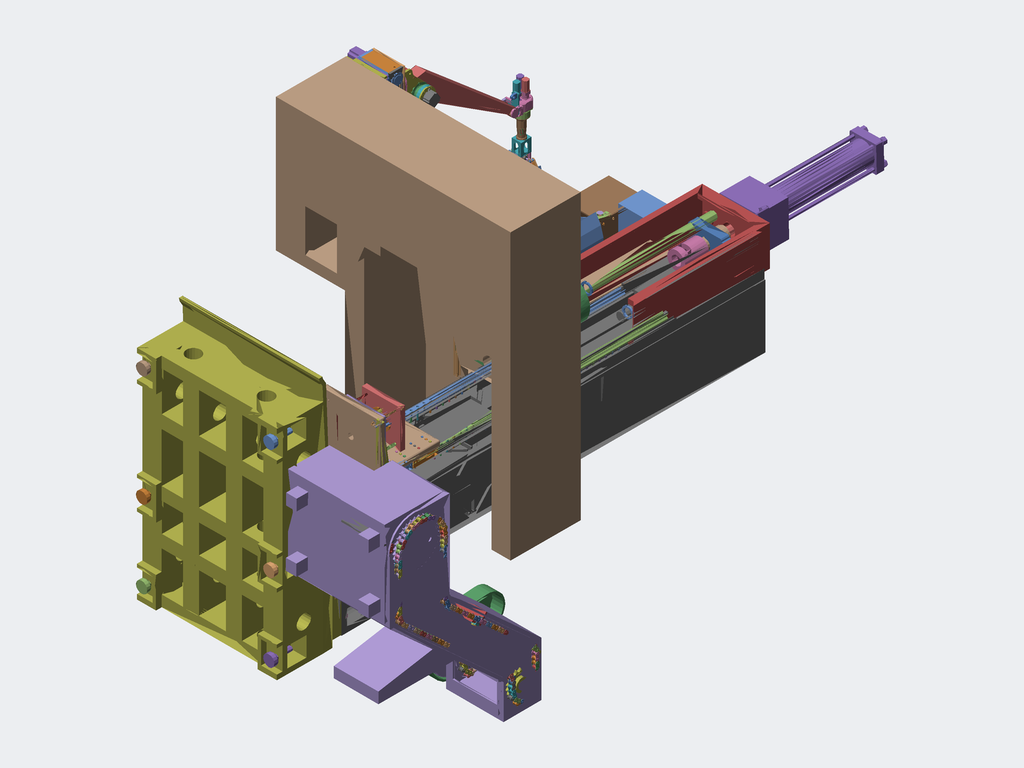Assembly | STEP file | 873 different items | 873 placed
Parts list (item | name | quantity | parent item | size | volume), first 207 of 873 items:
1 | 2026.6.15-Main Assembly图.sldasm-Part-1 (subassembly) | x1 | in Z2026.6.15-Main Assembly图 | 250 x 30 x 250 mm | 249270 mm3
2 | 2026.6.15-Main Assembly图.sldasm-Part-10 (subassembly) | x1 | in Z2026.6.15-Main Assembly图 | 190 x 5 x 190 mm | 28274 mm3
3 | 2026.6.15-Main Assembly图.sldasm-Part-100 (subassembly) | x1 | in Z2026.6.15-Main Assembly图 | 10.629 x 36.003 x 36.231 mm | 7922 mm3
4 | 2026.6.15-Main Assembly图.sldasm-Part-101 (subassembly) | x1 | in Z2026.6.15-Main Assembly图 | 28.549 x 67.5 x 67.614 mm | 30514 mm3
5 | 2026.6.15-Main Assembly图.sldasm-Part-102 (subassembly) | x1 | in Z2026.6.15-Main Assembly图 | 34 x 34 x 6 mm | 3057 mm3
6 | 2026.6.15-Main Assembly图.sldasm-Part-103 (subassembly) | x1 | in Z2026.6.15-Main Assembly图 | 195 x 12 x 225 mm | 287509 mm3
7 | 2026.6.15-Main Assembly图.sldasm-Part-104 (subassembly) | x1 | in Z2026.6.15-Main Assembly图 | 22 x 70 x 70 mm | 36230 mm3
8 | 2026.6.15-Main Assembly图.sldasm-Part-105 (subassembly) | x1 | in Z2026.6.15-Main Assembly图 | 47.5 x 47.5 x 16 mm | 7161 mm3
9 | 2026.6.15-Main Assembly图.sldasm-Part-106 (subassembly) | x1 | in Z2026.6.15-Main Assembly图 | 30.153 x 30.153 x 77.25 mm | 50923 mm3
10 | 2026.6.15-Main Assembly图.sldasm-Part-107 (subassembly) | x1 | in Z2026.6.15-Main Assembly图 | 57.5 x 10 x 57.5 mm | 14891 mm3
11 | 2026.6.15-Main Assembly图.sldasm-Part-108 (subassembly) | x1 | in Z2026.6.15-Main Assembly图 | 170.9 x 80.5 x 7 mm | 96302 mm3
12 | 2026.6.15-Main Assembly图.sldasm-Part-109 (subassembly) | x1 | in Z2026.6.15-Main Assembly图 | 16.509 x 47.502 x 47.64 mm | 9532 mm3
13 | 2026.6.15-Main Assembly图.sldasm-Part-11 (subassembly) | x1 | in Z2026.6.15-Main Assembly图 | 23 x 23.6 x 790 mm | 320754 mm3
14 | 2026.6.15-Main Assembly图.sldasm-Part-110 (subassembly) | x1 | in Z2026.6.15-Main Assembly图 | 26 x 65 x 65 mm | 35291 mm3
15 | 2026.6.15-Main Assembly图.sldasm-Part-111 (subassembly) | x1 | in Z2026.6.15-Main Assembly图 | 7.5 x 7.5 x 53.995 mm | 2283 mm3
16 | 2026.6.15-Main Assembly图.sldasm-Part-112 (subassembly) | x1 | in Z2026.6.15-Main Assembly图 | 10 x 10 x 132.905 mm | 5947 mm3
17 | 2026.6.15-Main Assembly图.sldasm-Part-113 (subassembly) | x1 | in Z2026.6.15-Main Assembly图 | 98.5 x 65 x 65 mm | 266939 mm3
18 | 2026.6.15-Main Assembly图.sldasm-Part-114 (subassembly) | x1 | in Z2026.6.15-Main Assembly图 | 8.754 x 35.047 x 35.043 mm | 2415 mm3
19 | 2026.6.15-Main Assembly图.sldasm-Part-115 (subassembly) | x1 | in Z2026.6.15-Main Assembly图 | 195 x 11.5 x 180 mm | 198792 mm3
20 | 2026.6.15-Main Assembly图.sldasm-Part-116 (subassembly) | x1 | in Z2026.6.15-Main Assembly图 | 34 x 34 x 6 mm | 3057 mm3
21 | 2026.6.15-Main Assembly图.sldasm-Part-117 (subassembly) | x1 | in Z2026.6.15-Main Assembly图 | 235 x 45 x 265 mm | 353113 mm3
22 | 2026.6.15-Main Assembly图.sldasm-Part-118 (subassembly) | x1 | in Z2026.6.15-Main Assembly图 | 52.5 x 52.5 x 6 mm | 2953 mm3
23 | 2026.6.15-Main Assembly图.sldasm-Part-119 (subassembly) | x1 | in Z2026.6.15-Main Assembly图 | 134.9 x 50 x 134.9 mm | 194237 mm3
24 | 2026.6.15-Main Assembly图.sldasm-Part-12 (subassembly) | x1 | in Z2026.6.15-Main Assembly图 | 14.453 x 75.3 x 14.544 mm | 4272 mm3
25 | 2026.6.15-Main Assembly图.sldasm-Part-120 (subassembly) | x1 | in Z2026.6.15-Main Assembly图 | 14.16 x 14.195 x 23.5 mm | 1185 mm3
26 | 2026.6.15-Main Assembly图.sldasm-Part-121 (subassembly) | x1 | in Z2026.6.15-Main Assembly图 | 16 x 16 x 4.5 mm | 703.994 mm3
27 | 2026.6.15-Main Assembly图.sldasm-Part-122 (subassembly) | x1 | in Z2026.6.15-Main Assembly图 | 15.533 x 56.283 x 47.914 mm | 23654 mm3
28 | 2026.6.15-Main Assembly图.sldasm-Part-123 (subassembly) | x1 | in Z2026.6.15-Main Assembly图 | 95 x 7 x 95 mm | 7521 mm3
29 | 2026.6.15-Main Assembly图.sldasm-Part-124 (subassembly) | x1 | in Z2026.6.15-Main Assembly图 | 67.5 x 8.5 x 67.5 mm | 21029 mm3
30 | 2026.6.15-Main Assembly图.sldasm-Part-125 (subassembly) | x1 | in Z2026.6.15-Main Assembly图 | 71.498 x 105 x 105.143 mm | 201131 mm3
31 | 2026.6.15-Main Assembly图.sldasm-Part-126 (subassembly) | x1 | in Z2026.6.15-Main Assembly图 | 120 x 19 x 120 mm | 119313 mm3
32 | 2026.6.15-Main Assembly图.sldasm-Part-127 (subassembly) | x1 | in Z2026.6.15-Main Assembly图 | 155 x 33 x 155 mm | 174909 mm3
33 | 2026.6.15-Main Assembly图.sldasm-Part-128 (subassembly) | x1 | in Z2026.6.15-Main Assembly图 | 12.5 x 12.5 x 26.5 mm | 1705 mm3
34 | 2026.6.15-Main Assembly图.sldasm-Part-129 (subassembly) | x1 | in Z2026.6.15-Main Assembly图 | 105.045 x 102.69 x 47.501 mm | 174792 mm3
35 | 2026.6.15-Main Assembly图.sldasm-Part-13 (subassembly) | x1 | in Z2026.6.15-Main Assembly图 | 26.787 x 25.205 x 65.773 mm | 14698 mm3
36 | 2026.6.15-Main Assembly图.sldasm-Part-130 (subassembly) | x1 | in Z2026.6.15-Main Assembly图 | 32.571 x 17.473 x 17.472 mm | 4708 mm3
37 | 2026.6.15-Main Assembly图.sldasm-Part-131 (subassembly) | x1 | in Z2026.6.15-Main Assembly图 | 57.5 x 10 x 57.5 mm | 14891 mm3
38 | 2026.6.15-Main Assembly图.sldasm-Part-132 (subassembly) | x1 | in Z2026.6.15-Main Assembly图 | 21.6 x 102 x 102.517 mm | 128530 mm3
39 | 2026.6.15-Main Assembly图.sldasm-Part-133 (subassembly) | x1 | in Z2026.6.15-Main Assembly图 | 195.75 x 32 x 32 mm | 119299 mm3
40 | 2026.6.15-Main Assembly图.sldasm-Part-134 (subassembly) | x1 | in Z2026.6.15-Main Assembly图 | 82.035 x 635.638 x 507.509 mm | 499419 mm3
41 | 2026.6.15-Main Assembly图.sldasm-Part-135 (subassembly) | x1 | in Z2026.6.15-Main Assembly图 | 92.5 x 105 x 107.949 mm | 212796 mm3
42 | 2026.6.15-Main Assembly图.sldasm-Part-136 (subassembly) | x1 | in Z2026.6.15-Main Assembly图 | 7.5 x 107.5 x 103 mm | 13755 mm3
43 | 2026.6.15-Main Assembly图.sldasm-Part-137 (subassembly) | x1 | in Z2026.6.15-Main Assembly图 | 195 x 12 x 225 mm | 457954 mm3
44 | 2026.6.15-Main Assembly图.sldasm-Part-138 (subassembly) | x1 | in Z2026.6.15-Main Assembly图 | 170.9 x 80.5 x 7 mm | 95752 mm3
45 | 2026.6.15-Main Assembly图.sldasm-Part-139 (subassembly) | x1 | in Z2026.6.15-Main Assembly图 | 67.5 x 8.5 x 67.5 mm | 21029 mm3
46 | 2026.6.15-Main Assembly图.sldasm-Part-14 (subassembly) | x1 | in Z2026.6.15-Main Assembly图 | 13.397 x 75.3 x 14.988 mm | 4272 mm3
47 | 2026.6.15-Main Assembly图.sldasm-Part-140 (subassembly) | x1 | in Z2026.6.15-Main Assembly图 | 10 x 10 x 10 mm | 523.599 mm3
48 | 2026.6.15-Main Assembly图.sldasm-Part-141 (subassembly) | x1 | in Z2026.6.15-Main Assembly图 | 50 x 104.5 x 100 mm | 32634 mm3
49 | 2026.6.15-Main Assembly图.sldasm-Part-142 (subassembly) | x1 | in Z2026.6.15-Main Assembly图 | 64.6 x 81.962 x 82.084 mm | 155159 mm3
50 | 2026.6.15-Main Assembly图.sldasm-Part-143 (subassembly) | x1 | in Z2026.6.15-Main Assembly图 | 12 x 80.5 x 225 mm | 195559 mm3
51 | 2026.6.15-Main Assembly图.sldasm-Part-144 (subassembly) | x1 | in Z2026.6.15-Main Assembly图 | 10.798 x 102 x 102.145 mm | 33230 mm3
52 | 2026.6.15-Main Assembly图.sldasm-Part-145 (subassembly) | x1 | in Z2026.6.15-Main Assembly图 | 77.037 x 7.893 x 115 mm | 47591 mm3
53 | 2026.6.15-Main Assembly图.sldasm-Part-146 (subassembly) | x1 | in Z2026.6.15-Main Assembly图 | 30.153 x 30.153 x 57 mm | 33186 mm3
54 | 2026.6.15-Main Assembly图.sldasm-Part-147 (subassembly) | x1 | in Z2026.6.15-Main Assembly图 | 62.5 x 62.5 x 9 mm | 13262 mm3
55 | 2026.6.15-Main Assembly图.sldasm-Part-148 (subassembly) | x1 | in Z2026.6.15-Main Assembly图 | 90.222 x 100 x 48.5 mm | 102684 mm3
56 | 2026.6.15-Main Assembly图.sldasm-Part-149 (subassembly) | x1 | in Z2026.6.15-Main Assembly图 | 50 x 50 x 25 mm | 9308 mm3
57 | 2026.6.15-Main Assembly图.sldasm-Part-15 (subassembly) | x1 | in Z2026.6.15-Main Assembly图 | 27.711 x 45 x 24.161 mm | 11185 mm3
58 | 2026.6.15-Main Assembly图.sldasm-Part-150 (subassembly) | x1 | in Z2026.6.15-Main Assembly图 | 16 x 16 x 4.5 mm | 703.994 mm3
59 | 2026.6.15-Main Assembly图.sldasm-Part-151 (subassembly) | x1 | in Z2026.6.15-Main Assembly图 | 10.798 x 102 x 102.145 mm | 33230 mm3
60 | 2026.6.15-Main Assembly图.sldasm-Part-152 (subassembly) | x1 | in Z2026.6.15-Main Assembly图 | 34 x 34 x 6 mm | 3057 mm3
61 | 2026.6.15-Main Assembly图.sldasm-Part-153 (subassembly) | x1 | in Z2026.6.15-Main Assembly图 | 6.837 x 84.5 x 56.57 mm | 12087 mm3
62 | 2026.6.15-Main Assembly图.sldasm-Part-154 (subassembly) | x1 | in Z2026.6.15-Main Assembly图 | 90.202 x 35 x 10.539 mm | 23036 mm3
63 | 2026.6.15-Main Assembly图.sldasm-Part-155 (subassembly) | x1 | in Z2026.6.15-Main Assembly图 | 30.153 x 30.153 x 77.25 mm | 50923 mm3
64 | 2026.6.15-Main Assembly图.sldasm-Part-156 (subassembly) | x1 | in Z2026.6.15-Main Assembly图 | 14.5 x 14.5 x 38 mm | 3109 mm3
65 | 2026.6.15-Main Assembly图.sldasm-Part-157 (subassembly) | x1 | in Z2026.6.15-Main Assembly图 | 30.153 x 30.153 x 57 mm | 32608 mm3
66 | 2026.6.15-Main Assembly图.sldasm-Part-158 (subassembly) | x1 | in Z2026.6.15-Main Assembly图 | 87.5 x 166 x 87.5 mm | 296087 mm3
67 | 2026.6.15-Main Assembly图.sldasm-Part-159 (subassembly) | x1 | in Z2026.6.15-Main Assembly图 | 34 x 34 x 6 mm | 3057 mm3
68 | 2026.6.15-Main Assembly图.sldasm-Part-16 (subassembly) | x1 | in Z2026.6.15-Main Assembly图 | 600 x 60 x 600 mm | 8563551 mm3
69 | 2026.6.15-Main Assembly图.sldasm-Part-160 (subassembly) | x1 | in Z2026.6.15-Main Assembly图 | 57 x 66 x 81 mm | 71126 mm3
70 | 2026.6.15-Main Assembly图.sldasm-Part-161 (subassembly) | x1 | in Z2026.6.15-Main Assembly图 | 7.316 x 10.32 x 10.946 mm | 145.813 mm3
71 | 2026.6.15-Main Assembly图.sldasm-Part-162 (subassembly) | x1 | in Z2026.6.15-Main Assembly图 | 9.094 x 15.6 x 16.059 mm | 200.393 mm3
72 | 2026.6.15-Main Assembly图.sldasm-Part-163 (subassembly) | x1 | in Z2026.6.15-Main Assembly图 | 18 x 1.5 x 18 mm | 354.56 mm3
73 | 2026.6.15-Main Assembly图.sldasm-Part-164 (subassembly) | x1 | in Z2026.6.15-Main Assembly图 | 150 x 6 x 58.455 mm | 22886 mm3
74 | 2026.6.15-Main Assembly图.sldasm-Part-165 (subassembly) | x1 | in Z2026.6.15-Main Assembly图 | 2.381 x 2.381 x 2.381 mm | 7.071 mm3
75 | 2026.6.15-Main Assembly图.sldasm-Part-166 (subassembly) | x1 | in Z2026.6.15-Main Assembly图 | 23.4 x 7.5 x 16.8 mm | 1292 mm3
76 | 2026.6.15-Main Assembly图.sldasm-Part-167 (subassembly) | x1 | in Z2026.6.15-Main Assembly图 | 10.5 x 17.82 x 17.82 mm | 1584 mm3
77 | 2026.6.15-Main Assembly图.sldasm-Part-168 (subassembly) | x1 | in Z2026.6.15-Main Assembly图 | 2.381 x 2.381 x 2.381 mm | 7.071 mm3
78 | 2026.6.15-Main Assembly图.sldasm-Part-169 (subassembly) | x1 | in Z2026.6.15-Main Assembly图 | 2.381 x 2.381 x 2.381 mm | 7.071 mm3
79 | 2026.6.15-Main Assembly图.sldasm-Part-17 (subassembly) | x1 | in Z2026.6.15-Main Assembly图 | 70 x 30.5 x 64.5 mm | 99534 mm3
80 | 2026.6.15-Main Assembly图.sldasm-Part-170 (subassembly) | x1 | in Z2026.6.15-Main Assembly图 | 4.523 x 13.89 x 13.187 mm | 10.033 mm3
81 | 2026.6.15-Main Assembly图.sldasm-Part-171 (subassembly) | x1 | in Z2026.6.15-Main Assembly图 | 150 x 6 x 58.455 mm | 22886 mm3
82 | 2026.6.15-Main Assembly图.sldasm-Part-172 (subassembly) | x1 | in Z2026.6.15-Main Assembly图 | 5.989 x 9.6 x 6.551 mm | 119.337 mm3
83 | 2026.6.15-Main Assembly图.sldasm-Part-173 (subassembly) | x1 | in Z2026.6.15-Main Assembly图 | 6.92 x 7.621 x 7.885 mm | 95.325 mm3
84 | 2026.6.15-Main Assembly图.sldasm-Part-174 (subassembly) | x1 | in Z2026.6.15-Main Assembly图 | 2.343 x 21 x 21 mm | 106.322 mm3
85 | 2026.6.15-Main Assembly图.sldasm-Part-175 (subassembly) | x1 | in Z2026.6.15-Main Assembly图 | 30.721 x 36 x 29.365 mm | 11937 mm3
86 | 2026.6.15-Main Assembly图.sldasm-Part-176 (subassembly) | x1 | in Z2026.6.15-Main Assembly图 | 2.381 x 2.381 x 2.381 mm | 7.071 mm3
87 | 2026.6.15-Main Assembly图.sldasm-Part-177 (subassembly) | x1 | in Z2026.6.15-Main Assembly图 | 4.523 x 13.89 x 13.187 mm | 10.033 mm3
88 | 2026.6.15-Main Assembly图.sldasm-Part-178 (subassembly) | x1 | in Z2026.6.15-Main Assembly图 | 6.6 x 4.8 x 6.6 mm | 118.747 mm3
89 | 2026.6.15-Main Assembly图.sldasm-Part-179 (subassembly) | x1 | in Z2026.6.15-Main Assembly图 | 2.381 x 2.381 x 2.381 mm | 7.071 mm3
90 | 2026.6.15-Main Assembly图.sldasm-Part-18 (subassembly) | x1 | in Z2026.6.15-Main Assembly图 | 48 x 29.585 x 3.015 mm | 1583 mm3
91 | 2026.6.15-Main Assembly图.sldasm-Part-180 (subassembly) | x1 | in Z2026.6.15-Main Assembly图 | 9.599 x 2.798 x 8.476 mm | 26.852 mm3
92 | 2026.6.15-Main Assembly图.sldasm-Part-181 (subassembly) | x1 | in Z2026.6.15-Main Assembly图 | 9.599 x 2.798 x 8.476 mm | 26.852 mm3
93 | 2026.6.15-Main Assembly图.sldasm-Part-182 (subassembly) | x1 | in Z2026.6.15-Main Assembly图 | 18 x 24 x 18 mm | 5067 mm3
94 | 2026.6.15-Main Assembly图.sldasm-Part-183 (subassembly) | x1 | in Z2026.6.15-Main Assembly图 | 9.094 x 15.6 x 16.059 mm | 200.393 mm3
95 | 2026.6.15-Main Assembly图.sldasm-Part-184 (subassembly) | x1 | in Z2026.6.15-Main Assembly图 | 2.381 x 2.381 x 2.381 mm | 7.071 mm3
96 | 2026.6.15-Main Assembly图.sldasm-Part-185 (subassembly) | x1 | in Z2026.6.15-Main Assembly图 | 2.381 x 2.381 x 2.381 mm | 7.071 mm3
97 | 2026.6.15-Main Assembly图.sldasm-Part-186 (subassembly) | x1 | in Z2026.6.15-Main Assembly图 | 13.86 x 27 x 13.86 mm | 2333 mm3
98 | 2026.6.15-Main Assembly图.sldasm-Part-187 (subassembly) | x1 | in Z2026.6.15-Main Assembly图 | 13.86 x 27 x 13.86 mm | 2333 mm3
99 | 2026.6.15-Main Assembly图.sldasm-Part-188 (subassembly) | x1 | in Z2026.6.15-Main Assembly图 | 18 x 24 x 18 mm | 5067 mm3
100 | 2026.6.15-Main Assembly图.sldasm-Part-189 (subassembly) | x1 | in Z2026.6.15-Main Assembly图 | 30.721 x 36 x 29.365 mm | 11937 mm3
101 | 2026.6.15-Main Assembly图.sldasm-Part-19 (subassembly) | x1 | in Z2026.6.15-Main Assembly图 | 48 x 29.881 x 12.525 mm | 13643 mm3
102 | 2026.6.15-Main Assembly图.sldasm-Part-190 (subassembly) | x1 | in Z2026.6.15-Main Assembly图 | 2.381 x 2.381 x 2.381 mm | 7.071 mm3
103 | 2026.6.15-Main Assembly图.sldasm-Part-191 (subassembly) | x1 | in Z2026.6.15-Main Assembly图 | 2.381 x 2.381 x 2.381 mm | 7.071 mm3
104 | 2026.6.15-Main Assembly图.sldasm-Part-192 (subassembly) | x1 | in Z2026.6.15-Main Assembly图 | 5.7 x 0.45 x 5.7 mm | 3.936 mm3
105 | 2026.6.15-Main Assembly图.sldasm-Part-193 (subassembly) | x1 | in Z2026.6.15-Main Assembly图 | 2.381 x 2.381 x 2.381 mm | 7.071 mm3
106 | 2026.6.15-Main Assembly图.sldasm-Part-194 (subassembly) | x1 | in Z2026.6.15-Main Assembly图 | 2.381 x 2.381 x 2.381 mm | 7.071 mm3
107 | 2026.6.15-Main Assembly图.sldasm-Part-195 (subassembly) | x1 | in Z2026.6.15-Main Assembly图 | 4.523 x 13.89 x 13.187 mm | 10.033 mm3
108 | 2026.6.15-Main Assembly图.sldasm-Part-196 (subassembly) | x1 | in Z2026.6.15-Main Assembly图 | 30 x 1.5 x 30 mm | 963.585 mm3
109 | 2026.6.15-Main Assembly图.sldasm-Part-197 (subassembly) | x1 | in Z2026.6.15-Main Assembly图 | 15 x 4.2 x 15 mm | 367.131 mm3
110 | 2026.6.15-Main Assembly图.sldasm-Part-198 (subassembly) | x1 | in Z2026.6.15-Main Assembly图 | 2.381 x 2.381 x 2.381 mm | 7.071 mm3
111 | 2026.6.15-Main Assembly图.sldasm-Part-199 (subassembly) | x1 | in Z2026.6.15-Main Assembly图 | 4.491 x 4.5 x 5.1 mm | 10.749 mm3
112 | 2026.6.15-Main Assembly图.sldasm-Part-2 (subassembly) | x1 | in Z2026.6.15-Main Assembly图 | 190 x 5 x 190 mm | 28274 mm3
113 | 2026.6.15-Main Assembly图.sldasm-Part-20 (subassembly) | x1 | in Z2026.6.15-Main Assembly图 | 48 x 29.881 x 12.525 mm | 13643 mm3
114 | 2026.6.15-Main Assembly图.sldasm-Part-200 (subassembly) | x1 | in Z2026.6.15-Main Assembly图 | 50.44 x 27 x 130.381 mm | 11515 mm3
115 | 2026.6.15-Main Assembly图.sldasm-Part-201 (subassembly) | x1 | in Z2026.6.15-Main Assembly图 | 50.44 x 27 x 130.381 mm | 11515 mm3
116 | 2026.6.15-Main Assembly图.sldasm-Part-202 (subassembly) | x1 | in Z2026.6.15-Main Assembly图 | 2.381 x 2.381 x 2.381 mm | 7.071 mm3
117 | 2026.6.15-Main Assembly图.sldasm-Part-203 (subassembly) | x1 | in Z2026.6.15-Main Assembly图 | 2.381 x 2.381 x 2.381 mm | 7.071 mm3
118 | 2026.6.15-Main Assembly图.sldasm-Part-204 (subassembly) | x1 | in Z2026.6.15-Main Assembly图 | 30 x 1.5 x 30 mm | 963.585 mm3
119 | 2026.6.15-Main Assembly图.sldasm-Part-205 (subassembly) | x1 | in Z2026.6.15-Main Assembly图 | 2.381 x 2.381 x 2.381 mm | 7.071 mm3
120 | 2026.6.15-Main Assembly图.sldasm-Part-206 (subassembly) | x1 | in Z2026.6.15-Main Assembly图 | 6.927 x 7.621 x 7.888 mm | 95.325 mm3
121 | 2026.6.15-Main Assembly图.sldasm-Part-207 (subassembly) | x1 | in Z2026.6.15-Main Assembly图 | 5.7 x 0.45 x 5.7 mm | 3.936 mm3
122 | 2026.6.15-Main Assembly图.sldasm-Part-208 (subassembly) | x1 | in Z2026.6.15-Main Assembly图 | 2.381 x 2.381 x 2.381 mm | 7.071 mm3
123 | 2026.6.15-Main Assembly图.sldasm-Part-209 (subassembly) | x1 | in Z2026.6.15-Main Assembly图 | 73.5 x 21 x 21 mm | 6492 mm3
124 | 2026.6.15-Main Assembly图.sldasm-Part-21 (subassembly) | x1 | in Z2026.6.15-Main Assembly图 | 48 x 29.585 x 4.175 mm | 4340 mm3
125 | 2026.6.15-Main Assembly图.sldasm-Part-210 (subassembly) | x1 | in Z2026.6.15-Main Assembly图 | 2.425 x 2.1 x 4.05 mm | 8.483 mm3
126 | 2026.6.15-Main Assembly图.sldasm-Part-211 (subassembly) | x1 | in Z2026.6.15-Main Assembly图 | 7.316 x 10.32 x 10.946 mm | 145.813 mm3
127 | 2026.6.15-Main Assembly图.sldasm-Part-212 (subassembly) | x1 | in Z2026.6.15-Main Assembly图 | 10.5 x 4.8 x 10.5 mm | 217.628 mm3
128 | 2026.6.15-Main Assembly图.sldasm-Part-213 (subassembly) | x1 | in Z2026.6.15-Main Assembly图 | 2.474 x 2.1 x 4.168 mm | 8.483 mm3
129 | 2026.6.15-Main Assembly图.sldasm-Part-214 (subassembly) | x1 | in Z2026.6.15-Main Assembly图 | 4.49 x 2.7 x 2.798 mm | 4.734 mm3
130 | 2026.6.15-Main Assembly图.sldasm-Part-215 (subassembly) | x1 | in Z2026.6.15-Main Assembly图 | 19.168 x 36 x 31.533 mm | 11937 mm3
131 | 2026.6.15-Main Assembly图.sldasm-Part-216 (subassembly) | x1 | in Z2026.6.15-Main Assembly图 | 2.381 x 2.381 x 2.381 mm | 7.071 mm3
132 | 2026.6.15-Main Assembly图.sldasm-Part-217 (subassembly) | x1 | in Z2026.6.15-Main Assembly图 | 18 x 1.5 x 18 mm | 354.56 mm3
133 | 2026.6.15-Main Assembly图.sldasm-Part-218 (subassembly) | x1 | in Z2026.6.15-Main Assembly图 | 2.381 x 2.381 x 2.381 mm | 7.071 mm3
134 | 2026.6.15-Main Assembly图.sldasm-Part-219 (subassembly) | x1 | in Z2026.6.15-Main Assembly图 | 2.343 x 21 x 21 mm | 106.322 mm3
135 | 2026.6.15-Main Assembly图.sldasm-Part-22 (subassembly) | x1 | in Z2026.6.15-Main Assembly图 | 48 x 29.585 x 4.175 mm | 4340 mm3
136 | 2026.6.15-Main Assembly图.sldasm-Part-220 (subassembly) | x1 | in Z2026.6.15-Main Assembly图 | 2.381 x 2.381 x 2.381 mm | 7.071 mm3
137 | 2026.6.15-Main Assembly图.sldasm-Part-221 (subassembly) | x1 | in Z2026.6.15-Main Assembly图 | 57 x 60 x 77.955 mm | 36451 mm3
138 | 2026.6.15-Main Assembly图.sldasm-Part-222 (subassembly) | x1 | in Z2026.6.15-Main Assembly图 | 15 x 20.7 x 20.7 mm | 3082 mm3
139 | 2026.6.15-Main Assembly图.sldasm-Part-223 (subassembly) | x1 | in Z2026.6.15-Main Assembly图 | 5.984 x 9.6 x 6.553 mm | 119.337 mm3
140 | 2026.6.15-Main Assembly图.sldasm-Part-224 (subassembly) | x1 | in Z2026.6.15-Main Assembly图 | 2.381 x 2.381 x 2.381 mm | 7.071 mm3
141 | 2026.6.15-Main Assembly图.sldasm-Part-225 (subassembly) | x1 | in Z2026.6.15-Main Assembly图 | 4.523 x 13.89 x 13.187 mm | 10.033 mm3
142 | 2026.6.15-Main Assembly图.sldasm-Part-226 (subassembly) | x1 | in Z2026.6.15-Main Assembly图 | 2.7 x 4.372 x 2.55 mm | 4.734 mm3
143 | 2026.6.15-Main Assembly图.sldasm-Part-227 (subassembly) | x1 | in Z2026.6.15-Main Assembly图 | 10.5 x 4.8 x 10.5 mm | 217.629 mm3
144 | 2026.6.15-Main Assembly图.sldasm-Part-228 (subassembly) | x1 | in Z2026.6.15-Main Assembly图 | 2.381 x 2.381 x 2.381 mm | 7.071 mm3
145 | 2026.6.15-Main Assembly图.sldasm-Part-229 (subassembly) | x1 | in Z2026.6.15-Main Assembly图 | 53.513 x 9.6 x 24.381 mm | 2422 mm3
146 | 2026.6.15-Main Assembly图.sldasm-Part-23 (subassembly) | x1 | in Z2026.6.15-Main Assembly图 | 14.821 x 7.8 x 14.088 mm | 645.564 mm3
147 | 2026.6.15-Main Assembly图.sldasm-Part-230 (subassembly) | x1 | in Z2026.6.15-Main Assembly图 | 18 x 1.5 x 18 mm | 354.56 mm3
148 | 2026.6.15-Main Assembly图.sldasm-Part-231 (subassembly) | x1 | in Z2026.6.15-Main Assembly图 | 6 x 39 x 15.045 mm | 2873 mm3
149 | 2026.6.15-Main Assembly图.sldasm-Part-232 (subassembly) | x1 | in Z2026.6.15-Main Assembly图 | 7.316 x 10.32 x 10.946 mm | 146.051 mm3
150 | 2026.6.15-Main Assembly图.sldasm-Part-233 (subassembly) | x1 | in Z2026.6.15-Main Assembly图 | 9.094 x 15.6 x 16.059 mm | 200.393 mm3
151 | 2026.6.15-Main Assembly图.sldasm-Part-234 (subassembly) | x1 | in Z2026.6.15-Main Assembly图 | 2.381 x 2.381 x 2.381 mm | 7.071 mm3
152 | 2026.6.15-Main Assembly图.sldasm-Part-235 (subassembly) | x1 | in Z2026.6.15-Main Assembly图 | 47.222 x 36 x 85.968 mm | 40942 mm3
153 | 2026.6.15-Main Assembly图.sldasm-Part-236 (subassembly) | x1 | in Z2026.6.15-Main Assembly图 | 3.9 x 8.4 x 3.9 mm | 52.478 mm3
154 | 2026.6.15-Main Assembly图.sldasm-Part-237 (subassembly) | x1 | in Z2026.6.15-Main Assembly图 | 10.41 x 3.004 x 9.59 mm | 44.117 mm3
155 | 2026.6.15-Main Assembly图.sldasm-Part-238 (subassembly) | x1 | in Z2026.6.15-Main Assembly图 | 78.583 x 4.5 x 190.718 mm | 23783 mm3
156 | 2026.6.15-Main Assembly图.sldasm-Part-239 (subassembly) | x1 | in Z2026.6.15-Main Assembly图 | 78.583 x 4.5 x 190.718 mm | 23783 mm3
157 | 2026.6.15-Main Assembly图.sldasm-Part-24 (subassembly) | x1 | in Z2026.6.15-Main Assembly图 | 48 x 29.585 x 3.015 mm | 1583 mm3
158 | 2026.6.15-Main Assembly图.sldasm-Part-240 (subassembly) | x1 | in Z2026.6.15-Main Assembly图 | 2.381 x 2.381 x 2.381 mm | 7.071 mm3
159 | 2026.6.15-Main Assembly图.sldasm-Part-241 (subassembly) | x1 | in Z2026.6.15-Main Assembly图 | 2.381 x 2.381 x 2.381 mm | 7.071 mm3
160 | 2026.6.15-Main Assembly图.sldasm-Part-242 (subassembly) | x1 | in Z2026.6.15-Main Assembly图 | 11.1 x 9.75 x 11.1 mm | 639.565 mm3
161 | 2026.6.15-Main Assembly图.sldasm-Part-243 (subassembly) | x1 | in Z2026.6.15-Main Assembly图 | 11.1 x 9.75 x 11.1 mm | 639.565 mm3
162 | 2026.6.15-Main Assembly图.sldasm-Part-244 (subassembly) | x1 | in Z2026.6.15-Main Assembly图 | 53.801 x 9.404 x 25.282 mm | 2422 mm3
163 | 2026.6.15-Main Assembly图.sldasm-Part-245 (subassembly) | x1 | in Z2026.6.15-Main Assembly图 | 82.8 x 9 x 9 mm | 4725 mm3
164 | 2026.6.15-Main Assembly图.sldasm-Part-246 (subassembly) | x1 | in Z2026.6.15-Main Assembly图 | 2.381 x 2.381 x 2.381 mm | 7.071 mm3
165 | 2026.6.15-Main Assembly图.sldasm-Part-247 (subassembly) | x1 | in Z2026.6.15-Main Assembly图 | 2.381 x 2.381 x 2.381 mm | 7.071 mm3
166 | 2026.6.15-Main Assembly图.sldasm-Part-248 (subassembly) | x1 | in Z2026.6.15-Main Assembly图 | 4.523 x 13.89 x 13.187 mm | 10.033 mm3
167 | 2026.6.15-Main Assembly图.sldasm-Part-249 (subassembly) | x1 | in Z2026.6.15-Main Assembly图 | 2.381 x 2.381 x 2.381 mm | 7.071 mm3
168 | 2026.6.15-Main Assembly图.sldasm-Part-25 (subassembly) | x1 | in Z2026.6.15-Main Assembly图 | 280 x 175 x 280 mm | 4284474 mm3
169 | 2026.6.15-Main Assembly图.sldasm-Part-250 (subassembly) | x1 | in Z2026.6.15-Main Assembly图 | 4.523 x 13.89 x 13.187 mm | 10.033 mm3
170 | 2026.6.15-Main Assembly图.sldasm-Part-251 (subassembly) | x1 | in Z2026.6.15-Main Assembly图 | 30 x 1.5 x 30 mm | 963.585 mm3
171 | 2026.6.15-Main Assembly图.sldasm-Part-252 (subassembly) | x1 | in Z2026.6.15-Main Assembly图 | 5.7 x 0.45 x 5.7 mm | 3.936 mm3
172 | 2026.6.15-Main Assembly图.sldasm-Part-253 (subassembly) | x1 | in Z2026.6.15-Main Assembly图 | 5.7 x 0.45 x 5.7 mm | 3.936 mm3
173 | 2026.6.15-Main Assembly图.sldasm-Part-254 (subassembly) | x1 | in Z2026.6.15-Main Assembly图 | 2.381 x 2.381 x 2.381 mm | 7.071 mm3
174 | 2026.6.15-Main Assembly图.sldasm-Part-255 (subassembly) | x1 | in Z2026.6.15-Main Assembly图 | 30.802 x 27 x 68.097 mm | 8755 mm3
175 | 2026.6.15-Main Assembly图.sldasm-Part-256 (subassembly) | x1 | in Z2026.6.15-Main Assembly图 | 30.802 x 27 x 68.097 mm | 8755 mm3
176 | 2026.6.15-Main Assembly图.sldasm-Part-257 (subassembly) | x1 | in Z2026.6.15-Main Assembly图 | 13.063 x 5.4 x 9.839 mm | 145.21 mm3
177 | 2026.6.15-Main Assembly图.sldasm-Part-258 (subassembly) | x1 | in Z2026.6.15-Main Assembly图 | 9.094 x 15.6 x 16.059 mm | 200.393 mm3
178 | 2026.6.15-Main Assembly图.sldasm-Part-259 (subassembly) | x1 | in Z2026.6.15-Main Assembly图 | 2.381 x 2.381 x 2.381 mm | 7.071 mm3
179 | 2026.6.15-Main Assembly图.sldasm-Part-26 (subassembly) | x1 | in Z2026.6.15-Main Assembly图 | 24.36 x 24 x 20.433 mm | 3958 mm3
180 | 2026.6.15-Main Assembly图.sldasm-Part-260 (subassembly) | x1 | in Z2026.6.15-Main Assembly图 | 2.381 x 2.381 x 2.381 mm | 7.071 mm3
181 | 2026.6.15-Main Assembly图.sldasm-Part-261 (subassembly) | x1 | in Z2026.6.15-Main Assembly图 | 11.1 x 0.45 x 11.081 mm | 15.053 mm3
182 | 2026.6.15-Main Assembly图.sldasm-Part-262 (subassembly) | x1 | in Z2026.6.15-Main Assembly图 | 6.6 x 4.8 x 6.6 mm | 118.747 mm3
183 | 2026.6.15-Main Assembly图.sldasm-Part-263 (subassembly) | x1 | in Z2026.6.15-Main Assembly图 | 11.1 x 9.75 x 11.1 mm | 639.565 mm3
184 | 2026.6.15-Main Assembly图.sldasm-Part-264 (subassembly) | x1 | in Z2026.6.15-Main Assembly图 | 11.1 x 9.75 x 11.1 mm | 639.565 mm3
185 | 2026.6.15-Main Assembly图.sldasm-Part-265 (subassembly) | x1 | in Z2026.6.15-Main Assembly图 | 10.07 x 9.6 x 11.459 mm | 173.019 mm3
186 | 2026.6.15-Main Assembly图.sldasm-Part-266 (subassembly) | x1 | in Z2026.6.15-Main Assembly图 | 2.381 x 2.381 x 2.381 mm | 7.071 mm3
187 | 2026.6.15-Main Assembly图.sldasm-Part-267 (subassembly) | x1 | in Z2026.6.15-Main Assembly图 | 2.381 x 2.381 x 2.381 mm | 7.071 mm3
188 | 2026.6.15-Main Assembly图.sldasm-Part-268 (subassembly) | x1 | in Z2026.6.15-Main Assembly图 | 30 x 1.5 x 30 mm | 963.585 mm3
189 | 2026.6.15-Main Assembly图.sldasm-Part-269 (subassembly) | x1 | in Z2026.6.15-Main Assembly图 | 4.523 x 13.89 x 13.187 mm | 10.033 mm3
190 | 2026.6.15-Main Assembly图.sldasm-Part-27 (subassembly) | x1 | in Z2026.6.15-Main Assembly图 | 24.36 x 24 x 20.433 mm | 3958 mm3
191 | 2026.6.15-Main Assembly图.sldasm-Part-270 (subassembly) | x1 | in Z2026.6.15-Main Assembly图 | 10.07 x 9.6 x 11.459 mm | 173.019 mm3
192 | 2026.6.15-Main Assembly图.sldasm-Part-271 (subassembly) | x1 | in Z2026.6.15-Main Assembly图 | 19.168 x 36 x 31.533 mm | 11937 mm3
193 | 2026.6.15-Main Assembly图.sldasm-Part-272 (subassembly) | x1 | in Z2026.6.15-Main Assembly图 | 7.316 x 10.32 x 10.946 mm | 146.017 mm3
194 | 2026.6.15-Main Assembly图.sldasm-Part-273 (subassembly) | x1 | in Z2026.6.15-Main Assembly图 | 78.583 x 4.5 x 190.718 mm | 23783 mm3
195 | 2026.6.15-Main Assembly图.sldasm-Part-274 (subassembly) | x1 | in Z2026.6.15-Main Assembly图 | 78.583 x 4.5 x 190.718 mm | 23783 mm3
196 | 2026.6.15-Main Assembly图.sldasm-Part-275 (subassembly) | x1 | in Z2026.6.15-Main Assembly图 | 47.222 x 36 x 85.968 mm | 40942 mm3
197 | 2026.6.15-Main Assembly图.sldasm-Part-276 (subassembly) | x1 | in Z2026.6.15-Main Assembly图 | 2.381 x 2.381 x 2.381 mm | 7.071 mm3
198 | 2026.6.15-Main Assembly图.sldasm-Part-277 (subassembly) | x1 | in Z2026.6.15-Main Assembly图 | 3.9 x 8.4 x 3.9 mm | 52.478 mm3
199 | 2026.6.15-Main Assembly图.sldasm-Part-278 (subassembly) | x1 | in Z2026.6.15-Main Assembly图 | 2.381 x 2.381 x 2.381 mm | 7.071 mm3
200 | 2026.6.15-Main Assembly图.sldasm-Part-279 (subassembly) | x1 | in Z2026.6.15-Main Assembly图 | 18 x 1.5 x 18 mm | 354.56 mm3
201 | 2026.6.15-Main Assembly图.sldasm-Part-28 (subassembly) | x1 | in Z2026.6.15-Main Assembly图 | 14.551 x 85.3 x 14.446 mm | 4774 mm3
202 | 2026.6.15-Main Assembly图.sldasm-Part-280 (subassembly) | x1 | in Z2026.6.15-Main Assembly图 | 13.066 x 5.4 x 9.826 mm | 145.21 mm3
203 | 2026.6.15-Main Assembly图.sldasm-Part-281 (subassembly) | x1 | in Z2026.6.15-Main Assembly图 | 4.486 x 4.5 x 5.098 mm | 10.749 mm3
204 | 2026.6.15-Main Assembly图.sldasm-Part-282 (subassembly) | x1 | in Z2026.6.15-Main Assembly图 | 3.6 x 21 x 21 mm | 1117 mm3
205 | 2026.6.15-Main Assembly图.sldasm-Part-283 (subassembly) | x1 | in Z2026.6.15-Main Assembly图 | 2.381 x 2.381 x 2.381 mm | 7.071 mm3
206 | 2026.6.15-Main Assembly图.sldasm-Part-284 (subassembly) | x1 | in Z2026.6.15-Main Assembly图 | 4.523 x 13.89 x 13.187 mm | 10.033 mm3
207 | 2026.6.15-Main Assembly图.sldasm-Part-285 (subassembly) | x1 | in Z2026.6.15-Main Assembly图 | 10.41 x 3.004 x 9.59 mm | 44.117 mm3